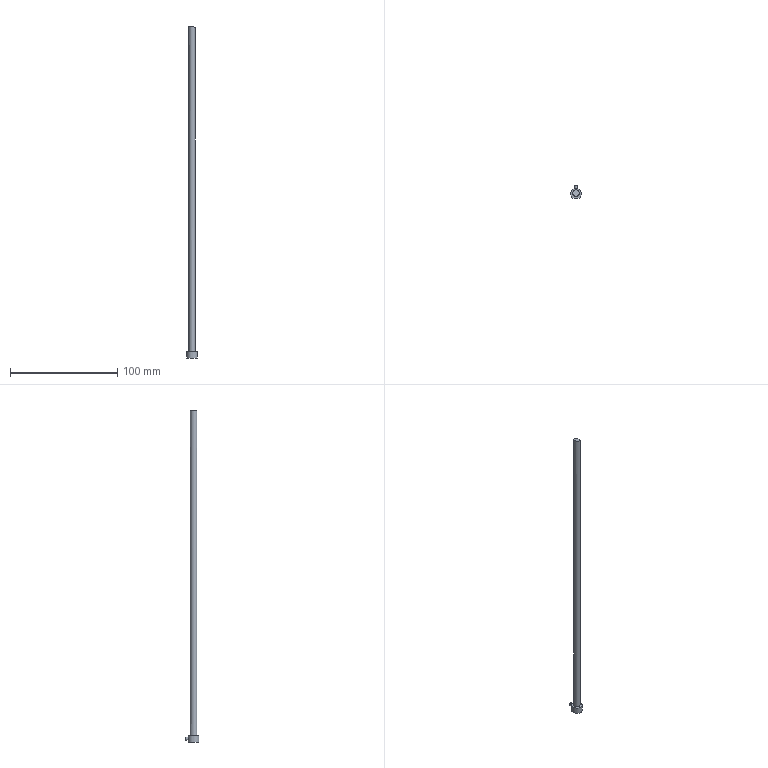Part | STEP file | E106-13-315 | 1 solid | 8 faces | box 10 x 13 x 309.676 mm | volume 9056 mm3 | cylinder 3 | plane 3 | spline 1 | cone 1 | commonest cylinder face diameters 3 x1 6 x1 10 x1